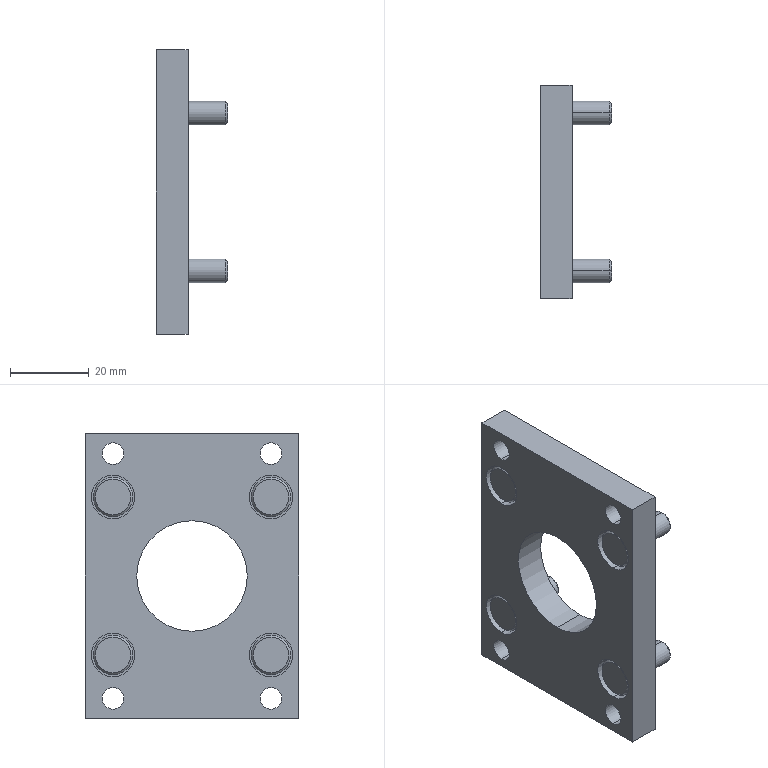Part | STEP file | _CDQ2F_40().stp | 1 solid | 80 faces | box 18 x 54 x 72 mm | volume 25983 mm3 | cylinder 42 | plane 22 | cone 16 | commonest cylinder face diameters 5.5 x8 6 x8 6.6 x8 10 x8 11 x8 28 x2